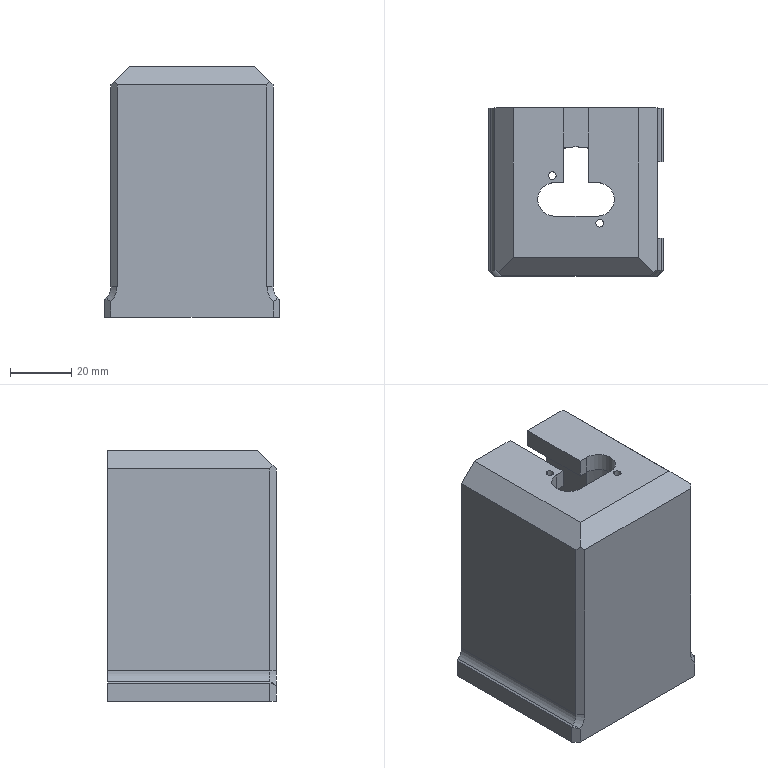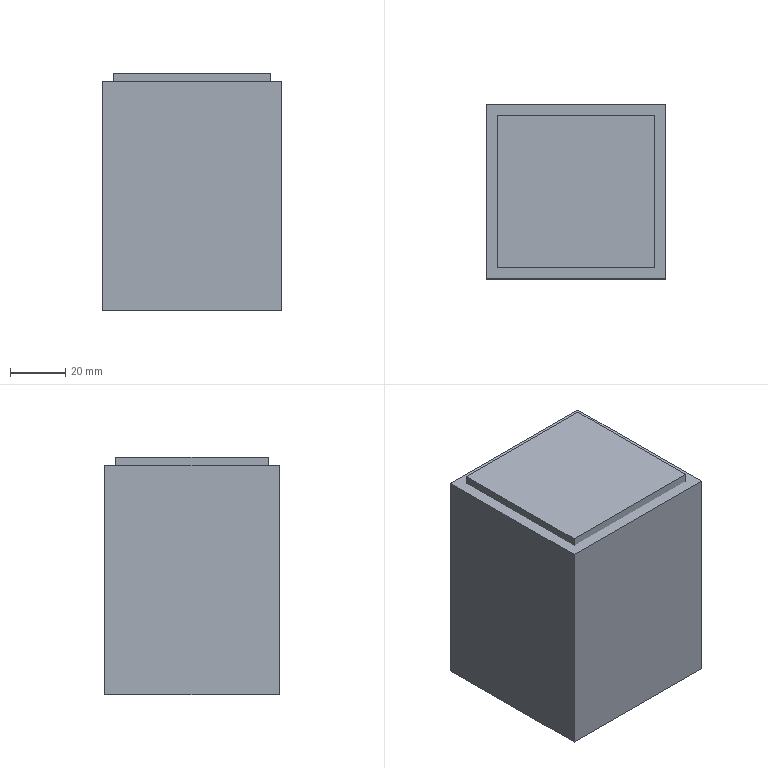CAM job | NX | 3-axis milling, drilling | part box 57 x 55 x 82 mm | stock box 65 x 63 x 86 mm
Tools:
number,name,description,diameter,corner_radius,flute_length,length,flutes
1,D63,Milling Tool-5 Parameters,63.0,0.0,50.0,75.0,2
7,D6A45,Milling Tool-5 Parameters,6.0,0.0,3.0,3.0,2
8,2.5ZT,Drilling Tool,2.5,0.0,35.0,50.0,2
9,M3,Milling Tool-5 Parameters,2.5,0.0,30.0,30.0,4
20,D20,Milling Tool-5 Parameters,20.0,0.0,50.0,75.0,2
6,D6,Milling Tool-5 Parameters,6.0,0.0,50.0,75.0,2
5,D6R0.5,Milling Tool-5 Parameters,6.0,0.5,50.0,75.0,2
12,2.8ZT,Drilling Tool,2.8,0.0,35.0,50.0,2
13,3.0JD,Milling Tool-5 Parameters,3.0,0.0,30.0,30.0,4
11,D10JING,Milling Tool-5 Parameters,10.0,0.0,50.0,75.0,2
Operations:
program,operation,operation_type,tool,method,geometry_group,spindle_rpm,surface_speed,feed_per_tooth,feed_cut,feed_plunge,cut_length_mm,path_length_mm,cut_time_min,machine_time_min
1-86-60-60毛胚,FLOOR_WALL,VolumeBased25DMillingOperation,D63,METHOD,A,6500.0,1286.0,0.0962,1250.0,100.0,305.797,359.797,0.2446,0.25
1-86-60-60毛胚,DRILLING_COPY_1,Operation,D6A45,METHOD,A,3000.0,56.0,0.0333,200.0,0.0,9.2,103.604,0.046,0.0554
1-86-60-60毛胚,DRILLING_COPY_1_COPY_1,Operation,2.5ZT,METHOD,A,2000.0,15.0,0.0375,150.0,0.0,22.502,130.208,0.15,0.1608
1-86-60-60毛胚,DRILLING_COPY_1_COPY_COPY_2,Operation,M3,METHOD,A,200.0,1.0,0.0006,0.5,0.0,19.0,123.204,38.0,38.01
1-86-60-60毛胚,ZLEVEL_PROFILE,ZLevelMilling,D20,METHOD,A,7000.0,439.0,0.1071,1500.0,1000.0,38022.868,38161.868,25.362,25.376
1-86-60-60毛胚,ZLEVEL_PROFILE_COPY_COPY_1,ZLevelMilling,D20,METHOD,A,7000.0,439.0,0.0571,800.0,100.0,1246.246,1492.634,1.558,1.582
1-86-60-60毛胚,ZLEVEL_PROFILE_COPY_COPY_1_COPY,ZLevelMilling,D20,METHOD,A,7000.0,439.0,0.0571,800.0,100.0,320.374,542.374,0.4005,0.4227
1-86-60-60毛胚,ZLEVEL_PROFILE_COPY_COPY_1_COPY_COPY,ZLevelMilling,D20,METHOD,A,7000.0,439.0,0.1429,2000.0,100.0,5023.724,5779.156,2.512,2.587
1-86-60-60毛胚,ZLEVEL_PROFILE_COPY_COPY_1_COPY_COPY_COPY,ZLevelMilling,D6,METHOD,A,7000.0,439.0,0.1429,2000.0,100.0,1229.689,1307.615,0.6148,0.6226
1-86-60-60毛胚,ZLEVEL_PROFILE_COPY_COPY_1_COPY_COPY_2_COPY_1,ZLevelMilling,D6R0.5,METHOD,A,7000.0,131.0,0.2143,3000.0,100.0,18900.769,18967.327,6.3,6.307
1-86-60-60毛胚,ZLEVEL_PROFILE_COPY_1_COPY_COPY_COPY_COPY_2_COPY,ZLevelMilling,D6A45,METHOD,A,7000.0,131.0,0.0714,1000.0,1000.0,148.803,210.803,0.1488,0.155
2-86-60-60毛胚,FLOOR_WALL_COPY,VolumeBased25DMillingOperation,D63,METHOD,B,6500.0,1286.0,0.0962,1250.0,100.0,1127.188,1420.58,0.9018,0.9311
2-86-60-60毛胚,DRILLING_COPY_1_COPY,Operation,D6A45,METHOD,B,3000.0,56.0,0.0333,200.0,0.0,27.6,262.965,0.138,0.1615
2-86-60-60毛胚,DRILLING_COPY_1_COPY_1_COPY,Operation,2.5ZT,METHOD,B,2000.0,15.0,0.0375,150.0,0.0,53.004,306.32,0.3534,0.3787
2-86-60-60毛胚,DRILLING_COPY_1_COPY_COPY_2_COPY,Operation,M3,METHOD,B,200.0,1.0,0.0006,0.5,0.0,50.0,300.311,100.0,100.025
2-86-60-60毛胚,DRILLING_COPY_1_COPY_1_COPY_COPY,Operation,2.8ZT,METHOD,B,2000.0,15.0,0.0375,150.0,0.0,22.0,156.092,0.1467,0.1601
2-86-60-60毛胚,DRILLING_COPY_1_COPY_1_COPY_COPY_COPY,Operation,3.0JD,METHOD,B,1000.0,9.0,0.01,40.0,0.0,22.0,156.092,0.55,0.5634
2-86-60-60毛胚,CAVITY_MILL,CavityMilling,D20,METHOD,B,7000.0,439.0,0.1571,2200.0,1000.0,17638.365,25852.899,10.457,11.297
2-86-60-60毛胚,ZLEVEL_PROFILE_COPY_COPY_1_1_COPY_COPY,ZLevelMilling,D20,METHOD,B,7000.0,439.0,0.0571,800.0,100.0,348.02,483.02,0.435,0.4485
2-86-60-60毛胚,ZLEVEL_PROFILE_COPY_COPY_1_1_COPY_COPY_COPY,ZLevelMilling,D20,METHOD,B,7000.0,439.0,0.0571,800.0,100.0,126.95,268.95,0.1587,0.1729
2-86-60-60毛胚,ZLEVEL_PROFILE_COPY_COPY_1_1_COPY_COPY_COPY_COPY,ZLevelMilling,D20,METHOD,B,7000.0,439.0,0.0571,800.0,100.0,122.422,334.224,0.153,0.1742
2-86-60-60毛胚,ZLEVEL_PROFILE_COPY_1,ZLevelMilling,D10JING,METHOD,B,7000.0,87.0,0.1071,1500.0,1000.0,5229.515,8654.829,3.802,4.144
2-86-60-60毛胚,FLOOR_WALL_1_COPY_1,VolumeBased25DMillingOperation,D10JING,METHOD,B,7000.0,87.0,0.0714,1000.0,100.0,433.513,791.718,0.4335,0.4725
2-86-60-60毛胚,ZLEVEL_PROFILE_COPY_COPY_1_COPY_COPY_COPY_1,ZLevelMilling,D10JING,METHOD,B,7000.0,439.0,0.1429,2000.0,100.0,1506.868,1804.291,0.7534,0.7832
2-86-60-60毛胚,ZLEVEL_PROFILE_COPY_1_COPY_COPY_COPY_COPY_2_COPY_COPY,ZLevelMilling,D6A45,METHOD,B,7000.0,131.0,0.0714,1000.0,1000.0,382.328,1054.938,0.3823,0.4496